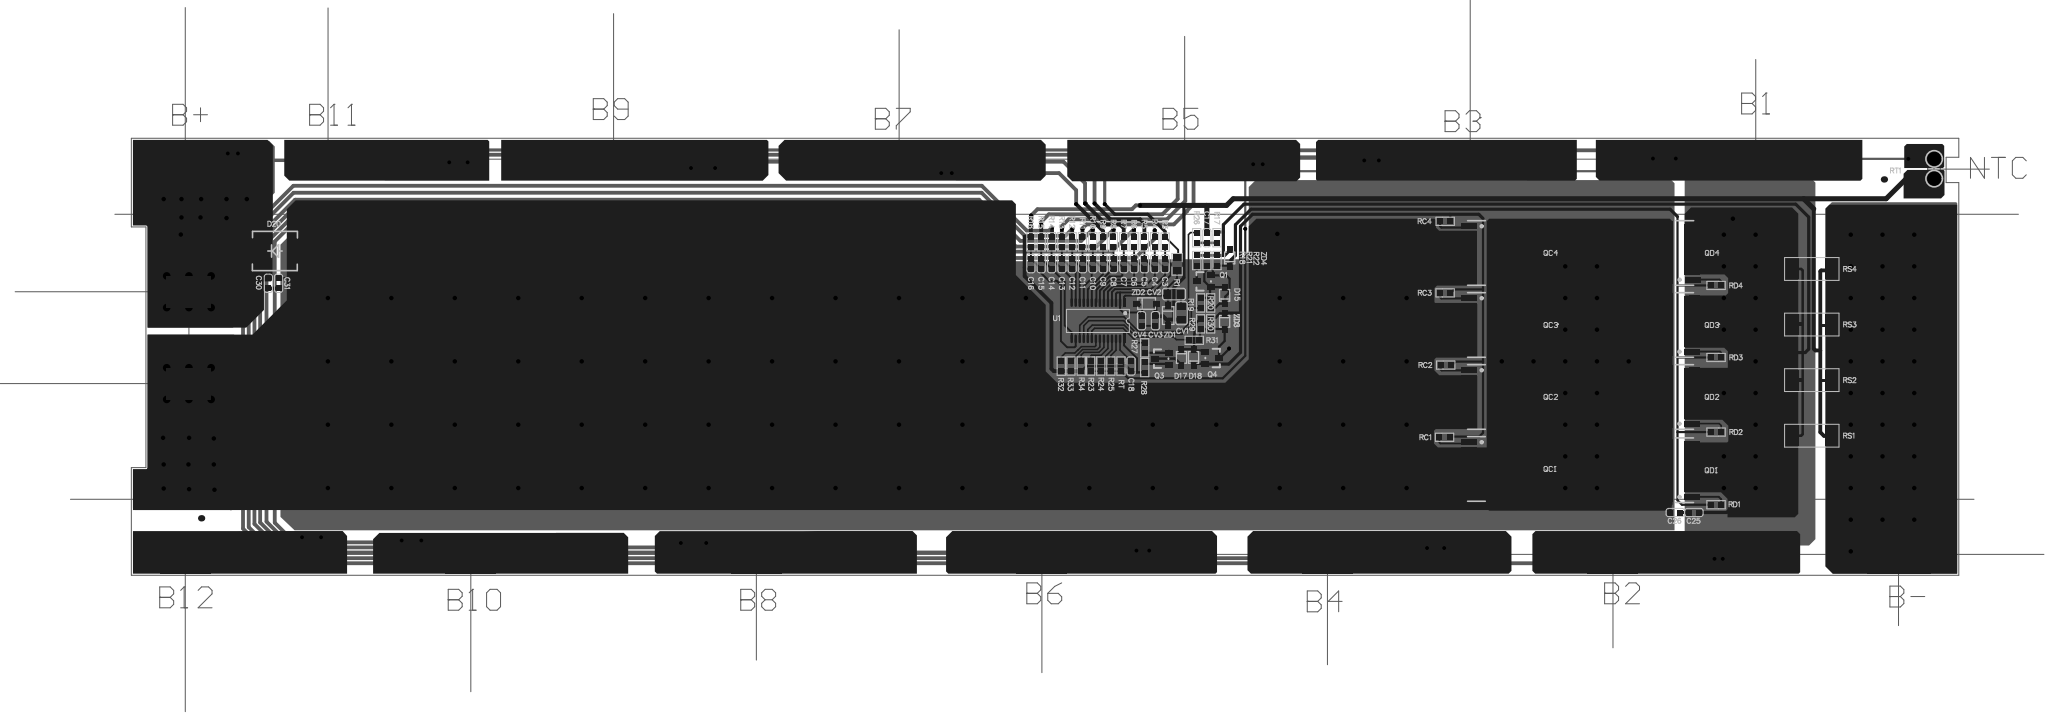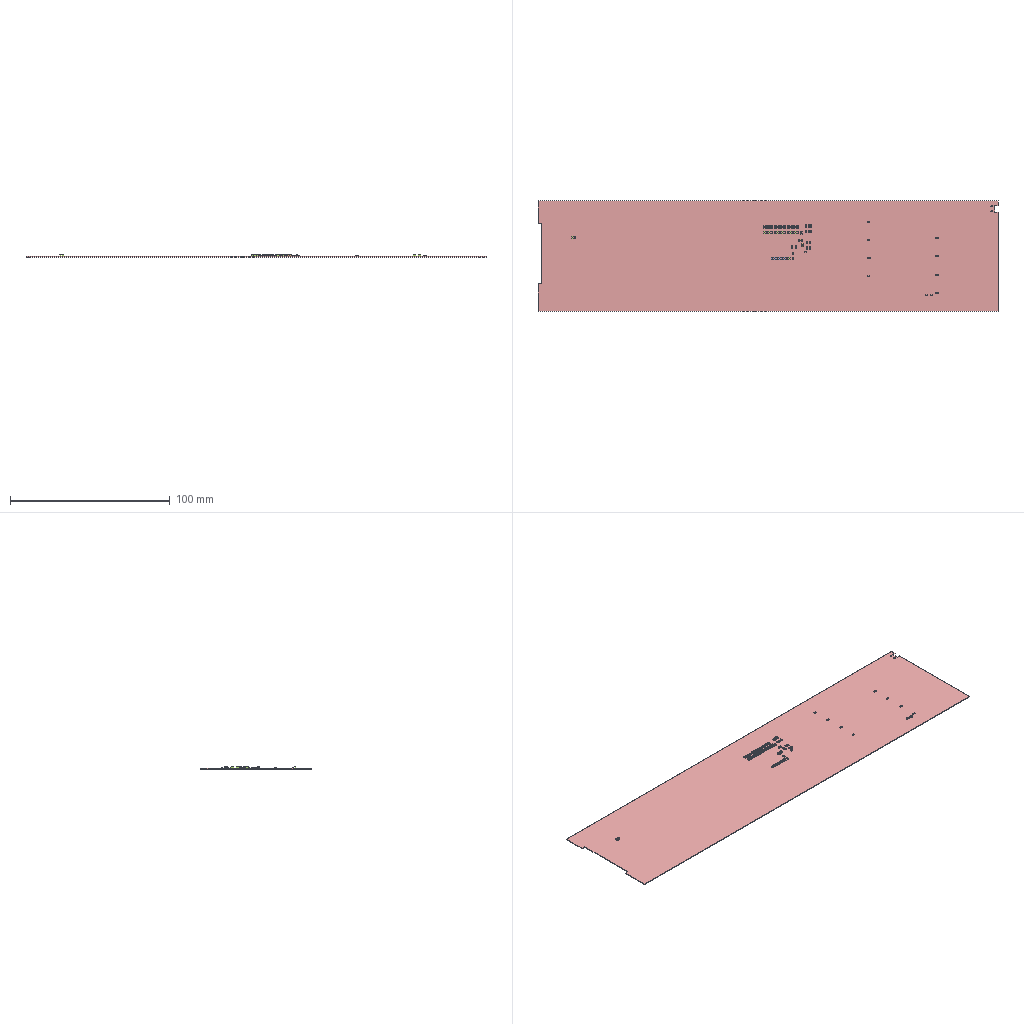Circuit board layout | Altium Designer | box 288 x 69 x 1.3 mm
Layer stack:
# Altium Designer layer stack of  (unit mm; dielectric type: 0 none, 1 core, 2 prepreg, 3 surface material)
index,name,kind,layer,copper_thickness_mm,dielectric_type,dielectric_thickness_mm,dielectric_material,dielectric_constant
0,Top Paste,other,,,,,,
1,Top Overlay,other,,,,,,
2,Top Solder,dielectric,,,3,0.0102,Solder Resist,3.5
3,Top Layer,copper,Top Layer,0.0356,,,,
4,Dielectric 1,dielectric,,,0,0.32,FR-4,4.8
5,Bottom Layer,copper,Bottom Layer,0.0356,,,,
6,Bottom Solder,dielectric,,,3,0.0102,Solder Resist,3.5
7,Bottom Overlay,other,,,,,,
8,Bottom Paste,other,,,,,,
# drill layer pairs: low layer,high layer
drill_pair,Top Layer,Bottom Layer
Part placement:
Designator,Comment,Layer,Footprint,Center-X(mm),Center-Y(mm),Rotation
ZD4,15V,TopLayer,SOD323,173.1,15.6,270
D15,1N4148,TopLayer,SOD323,172.3,9.7,270
QD1,NMOS,TopLayer,TOLL_123,242.643,-17.912,90
QD4,NMOS,TopLayer,TOLL_123,242.672,16.388,90
QD3,NMOS,TopLayer,TOLL_123,242.643,5.021,90
QD2,NMOS,TopLayer,TOLL_123,242.643,-6.349,90
QC3,NMOS,TopLayer,TOLL_123,214.133,5.021,270
QC2,NMOS,TopLayer,TOLL_123,214.133,-6.349,270
QC1,NMOS,TopLayer,TOLL_123,214.133,-17.712,270
QC4,NMOS,TopLayer,TOLL_123,214.133,16.388,270
ZD3,15V,TopLayer,SOD323,172.3,5.6,90
RT1,103AT B=3435,TopLayer,WK,284.117,29.69,270
RC4,47R,TopLayer,RES0603,207.055,21.388,270
RC3,47R,TopLayer,RES0603,207.045,10.088,270
RC2,47R,TopLayer,RES0603,207.145,-1.312,270
RC1,47R,TopLayer,RES0603,206.955,-12.712,270
R32,200K,TopLayer,RES0603,146.55,-1.482,0
ZD2,68V,TopLayer,SOD123,160,8.4,180
C15,104,TopLayer,CAP0603,143.395,14.7,0
C31,0.1uF,TopLayer,CAP0603,23.2,11.6,0
C30,0.1uF,TopLayer,CAP0603,21.6,11.6,180
RS4,,TopLayer,2512,264.845,13.863,90
RS3,,TopLayer,2512,264.845,5.088,90
RD4,47R,TopLayer,RES0603,249.745,11.263,90
RT,NC,TopLayer,RES0603,155.959,-1.467,180
R34,499K,TopLayer,RES0603,149.7,-1.457,0
RD3,47R,TopLayer,RES0603,249.745,-0.1123,90
RD2,47R,TopLayer,RES0603,249.745,-11.887,90
RD1,47R,TopLayer,RES0603,249.745,-23.362,90
R33,200K,TopLayer,RES0603,148.075,-1.457,0
R18,510R,TopLayer,RES0603,167.9,15.19,180
ZD1,68V,TopLayer,SOD123,163.4,6.5,90
U1,CW1143,TopLayer,SSOP-28-0.635,152.322,5.7,270
RS2,,TopLayer,2512,264.845,-3.687,90
RS1,,TopLayer,2512,264.845,-12.462,90
R31,1M,TopLayer,RES0603,167.51,2.6,90
R30,5.1M,TopLayer,RES0603,170.1,5.2,0
R29,5.1M,TopLayer,RES0603,168.5,5.2,0
R28,3M,TopLayer,RES0603,159.7,-1.7,180
R27,10K,TopLayer,RES0603,159.7,1.41,180
R25,22K,TopLayer,RES0603,154.368,-1.467,0
R24,41.2K,TopLayer,RES0603,152.776,-1.467,0
R23,270K,TopLayer,RES0603,151.185,-1.467,0
R22,5.1M,TopLayer,RES0603,171.1,15.2,180
R21,5.1M,TopLayer,RES0603,169.5,15.2,180
R20,NC,TopLayer,RES0603,170.1,8.5,0
R19,1K,TopLayer,RES0603,168.5,8.5,180
R26,10K,TopLayer,RES0603,167.9,18.8,180
R17,1K,TopLayer,RES0603,171.1,18.8,180
R16,2K,TopLayer,RES0603,141.767,18.15,0
R15,2K,TopLayer,RES0603,143.393,18.15,0
R14,2K,TopLayer,RES0603,145.019,18.15,0
R13,2K,TopLayer,RES0603,146.645,18.15,0
R12,2K,TopLayer,RES0603,148.27,18.15,0
R11,2K,TopLayer,RES0603,149.896,18.15,0
R10,2K,TopLayer,RES0603,151.522,18.15,0
R9,2K,TopLayer,RES0603,153.148,18.15,0
R8,2K,TopLayer,RES0603,154.774,18.15,0
R7,2K,TopLayer,RES0603,156.399,18.15,0
R6,2K,TopLayer,RES0603,158.025,18.15,0
R5,2K,TopLayer,RES0603,159.651,18.15,0
R4,2K,TopLayer,RES0603,161.277,18.15,0
R3,2K,TopLayer,RES0603,162.922,18.1,0
R1,2K,TopLayer,RES0805,164.8,14.584,270
Q4,MMBT5401,TopLayer,SOT-23-3,170.3,-0.2,270
Q3,MMBT5401,TopLayer,SOT-23-3,162.4,-0.3,90
Q1,MMBT5401,TopLayer,SOT-23-3,169.1,11.9,90
D20,RS3M,TopLayer,SMC,22.625,16.7,180
D18,1N4148,TopLayer,SOD323,167.4,-0.1,270
D17,1N4148,TopLayer,SOD323,165.5,-0.1,90
CV4,0.1uF,TopLayer,CAP0603,159.2,5.7,180
CV3,0.1uF,TopLayer,CAP0603,161.4,5.7,0
CV2,2.2uF,TopLayer,CAP0805,164.3,9.9,180
CV1,2.2uF,TopLayer,CAP0805,165.5,6.9,90
C26,0.1uF,TopLayer,CAP0603,243.32,-24.587,270
C25,0.1uF,TopLayer,CAP0603,246.255,-24.587,270
C18,104,TopLayer,CAP0603,157.55,-1.467,0
C17,104,TopLayer,CAP0603,169.5,18.8,180
C16,0.47uF,TopLayer,CAP0603,141.767,14.7,0
C14,104,TopLayer,CAP0603,145.022,14.7,0
C13,104,TopLayer,CAP0603,146.649,14.7,0
C12,104,TopLayer,CAP0603,148.276,14.7,0
C11,104,TopLayer,CAP0603,149.904,14.7,0
C10,104,TopLayer,CAP0603,151.531,14.7,0
C9,104,TopLayer,CAP0603,153.158,14.7,0
C8,104,TopLayer,CAP0603,154.786,14.7,0
C7,104,TopLayer,CAP0603,156.413,14.7,0
C6,104,TopLayer,CAP0603,158.04,14.7,0
C5,104,TopLayer,CAP0603,159.668,14.7,0
C4,104,TopLayer,CAP0603,161.295,14.7,0
C3,104,TopLayer,CAP0603,162.922,14.7,0
Pad and via stacks:
# Altium Designer via and pad stacks of  (unit mm). Each distinct definition once, with the count of objects using it.
# via: kind,start_layer,end_layer,hole_mm,diameter_mm,mode(0 simple;1 top-mid-bottom;2 full stack),diameter_per_layer,count,example_net
# pad: kind,layer,hole_mm,hole_type(0 round;1 square;2 slot),plating,top_size,top_shape(1 round;2 rect;3 octagon;9 rounded rect),mid_size,bottom_size,mode,footprint,size_per_layer,count,example
pad,Top Layer,0,0,plated,1x0.8,2,1x0.8,1x0.8,0,SOD323,,10,ZD4.2
pad,Top Layer,0,0,plated,0.83x0.88,2,0.83x0.88,0.83x0.88,0,CAP0603,,44,C3.1
pad,Top Layer,0,0,plated,1.27x1.016,2,1.27x1.016,1.27x1.016,0,RES0805,,2,R1.1
pad,Top Layer,0,0,plated,0.83x0.88,2,0.83x0.88,0.83x0.88,0,RES0603,,82,R3.2
pad,Top Layer,0,0,plated,9.9x8,2,9.9x8,9.9x8,0,TOLL_123,,8,QC4.3
pad,Top Layer,0,0,plated,0.8x8,2,0.8x8,0.8x8,0,TOLL_123,,8,QC4.2
pad,Top Layer,0,0,plated,1.7x0.8,2,1.7x0.8,1.7x0.8,0,TOLL_123,,56,QC4.2
pad,Top Layer,0,0,plated,2.5x0.8,2,2.5x0.8,2.5x0.8,0,TOLL_123,,8,QC4.1
pad,Top Layer,0,0,plated,2x3.2,2,2x3.2,2x3.2,0,2512,,8,RS1.1
pad,Top Layer,0,0,plated,1.4x0.4,1,1.4x0.4,1.4x0.4,0,SSOP-28-0.635,,26,U1.27
pad,Top Layer,0,0,plated,1.4x0.4,2,1.4x0.4,1.4x0.4,0,SSOP-28-0.635,,2,U1.28
pad,Top Layer,0,0,plated,0.9144x1.2,2,0.9144x1.2,0.9144x1.2,0,SOT-23-3,,9,Q3.3
pad,Top Layer,0,0,plated,8x6,2,8x6,8x6,0,,,12,609
pad,Top Layer,0,0,plated,3x3,1,3x3,3x3,0,,,14,641
pad,Top Layer,0,0,plated,10x6,2,10x6,10x6,0,,,2,597
pad,Top Layer,0,0,plated,1.27x1.1,2,1.27x1.1,1.27x1.1,0,CAP0805,,2,CV2.1
pad,Top Layer,0,0,plated,1.27x1.016,2,1.27x1.016,1.27x1.016,0,CAP0805,,2,CV2.2
pad,Top Layer,0,0,plated,2.44x3.62,2,2.44x3.62,2.44x3.62,0,SMC,,2,D20.1
pad,Top Layer,0,0,plated,1x0.8,2,1x0.8,1x0.8,0,SOD123,,4,ZD2.1
pad,Top Layer,0,0,plated,1x1,1,1x1,1x1,0,,,2,650
pad,Top Layer,0,0,plated,7x5,2,7x5,7x5,0,,,2,598
pad,Keep-Out Layer,0.075,0,plated,0.075x0.075,1,0.075x0.075,0.075x0.075,0,,,2,1
pad,Multi-Layer,1,0,plated,2.2x2.2,1,2.2x2.2,2.2x2.2,0,WK,,2,RT1.2
via,Top Layer,Bottom Layer,0.5,0.7,0,,152,P-
via,Top Layer,Bottom Layer,0.8,1.2,0,,14,P-
via,Top Layer,Bottom Layer,0.4,0.6,0,,44,B12
Copper pours:
name,layer,net,type(0 solid;1 hatched;2 none)
NETR23_2_L01_P093,Top Layer,NetR23_2,0
B-_L01_P092,Top Layer,B-,0
NONET_L-01_P-001,Top Layer,P-,0
B-_L01_P088,Top Layer,B-,0
NONET_L-01_P-001,Top Layer,B6,0
NONET_L-01_P-001,Top Layer,B2,0
NONET_L-01_P-001,Top Layer,B4,0
NONET_L-01_P-001,Top Layer,B8,0
NONET_L-01_P-001,Top Layer,B12,0
B+_L01_P081,Top Layer,B+,0
NONET_L-01_P-001,Top Layer,B7,0
NONET_L-01_P-001,Top Layer,B3,0
NONET_L-01_P-001,Top Layer,B1,0
NONET_L-01_P-001,Top Layer,B9,0
NONET_L-01_P-001,Top Layer,B5,0
NONET_L-01_P-001,Top Layer,B11,0
NONET_L-01_P-001,Top Layer,B10,0
NONET_L-01_P-001,Top Layer,P-,0
NONET_L-01_P-001,Top Layer,NetC25_1,0
P-_L02_P095,Bottom Layer,P-,0
B+_L02_P094,Bottom Layer,B+,0
P-_L02_P091,Bottom Layer,P-,0
NONET_L-01_P-001,Bottom Layer,NetC25_1,0
B-_L02_P089,Bottom Layer,B-,0
Design rules, without the lines most boards share:
# Altium Designer design rules of  (exported by Altium Designer, unit mm)
# columns: name | kind | enabled | priority | scope1 | scope2 | descriptor | typed fields (field=value)
Schematic Supply Nets | 41 | enabled | 1 | InNet('B-') | All | Supply Net(s)(InNet('B-')) |
NetAntennae | 56 | enabled | 1 | All | All | Net Antennae (Tolerance=0mm) (All) |
SilkToSilkClearance | 55 | enabled | 1 | All | All | Silk to Silk (Clearance=0.254mm) (All),(All) |
SilkToSolderMaskClearance | 54 | enabled | 1 | IsPad | All | Silk To Solder Mask (Clearance=0.254mm) (IsPad),(All) |
MinimumSolderMaskSliver | 53 | enabled | 1 | All | All | Minimum Solder Mask Sliver (Gap=0.254mm) (All),(All) |
HoleToHoleClearance | 52 | enabled | 1 | All | All | Hole To Hole Clearance (Gap=0.254mm) (All),(All) | gap=0.254
DiffPairsRouting | 51 | enabled | 1 | All | All | Differential Pairs Uncoupled Length using the Gap Constraints (Min=0.254mm) (Max=0.254mm) (Prefered=0.254mm)  and Width Constraints (Min=0.381mm) (Max=0.381mm) (Prefered=0.381mm) (All) |
HoleSize | 42 | enabled | 1 | All | All | Hole Size Constraint (Min=0.025mm) (Max=2.54mm) (All) |
Height | 50 | enabled | 1 | All | All | Height Constraint (Min=0mm) (Max=25.4mm) (Prefered=12.7mm) (All) | min_height=0 max_height=25.4
ComponentClearance | 24 | enabled | 1 | All | All | Component Clearance Constraint ( Horizontal Gap = 0.2mm, Vertical Gap = 0.254mm ) (All),(All)  | gap=0.2
SolderMaskExpansion | 13 | enabled | 1 | All | All | Solder Mask Expansion (Expansion =0.102mm) (All) | expansion=0.1016
PasteMaskExpansion | 14 | enabled | 1 | All | All | Paste Mask Expansion (Expansion =0mm) (All) | expansion=0
RoutingVias | 11 | enabled | 1 | All | All | Routing Via (MinHoleWidth=0.4mm) (MaxHoleWidth=0.4mm) (PreferredHoleWidth=0.4mm) (MinWidth=0.6mm) (MaxWidth=0.6mm) (PreferedWidth=0.6mm) (All) | via_min_hole=0.4 via_max_hole=0.4 via_preferred_diameter=0.6 via_preferred_hole=0.4
RoutingCorners | 10 | enabled | 1 | All | All | Routing Corners (Style=45-Degree) (Min Setback=2.54mm) (Max Setback=2.54mm) (All) |
Width | 2 | enabled | 1 | All | All | Width Constraint (Min=0.2mm) (Max=1mm) (Preferred=0.25mm) (All) |
PolygonConnect | 20 | enabled | 1 | All | All | Polygon Connect Rule(Direct Connect )(Conductor Width=0.254mm) (Relief Angle=90 Angle) (Entries=4) (Air Gap Width=0.254mm) (All),(All) | connect_style(0=relief,1=direct,2=none)=1 relief_conductor_width=0.254 relief_entries=4
PlaneClearance | 12 | enabled | 1 | All | All | Power Plane Clearance (Clearance =0.508mm) (All) | clearance=0.508
PlaneConnect | 6 | enabled | 1 | All | All | Power Plane Connect Rule(Relief Connect )(Expansion=0.508mm) (Conductor Width=0.254mm) (Air Gap=0.254mm) (Entries=4) (All) | relief_conductor_width=0.254 relief_entries=4 relief_expansion=0.508
Clearance | 0 | enabled | 1 | All | All | Clearance Constraint (Gap=0.2mm) (All),(All) | gap=0.2